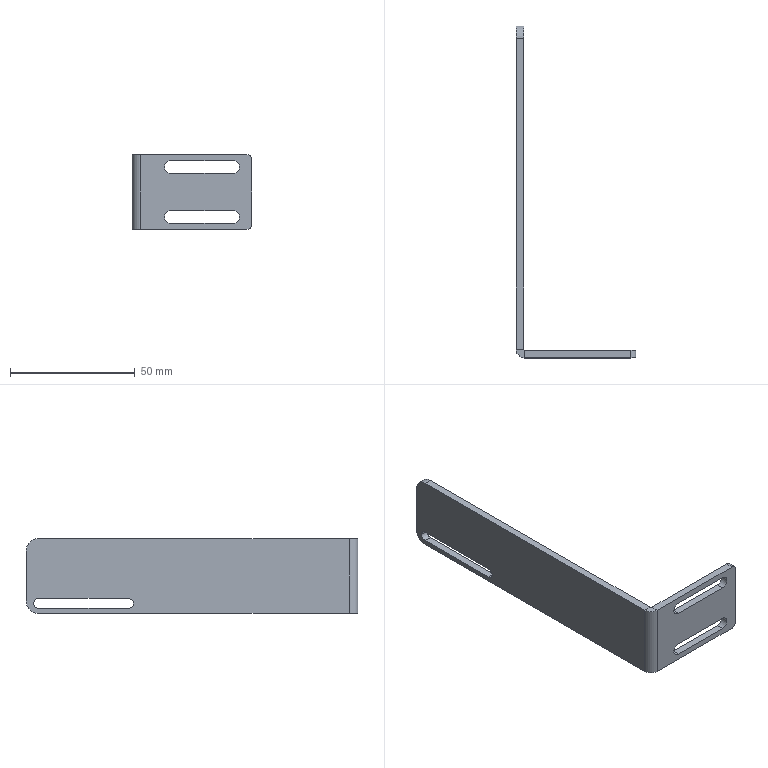Part | SolidWorks | features CornerTrim 2, ICE 2, FlatPattern 1, HoleWzd 1, SMBaseFlange 1, SheetMetal 1 | 1 solid | 31 faces | box 48 x 133 x 30 mm | volume 14568 mm3 | plane 18 | cylinder 13 | commonest cylinder face diameters 4 x5 5 x4 10 x2 1 x1 7 x1
STEP:
#1=CARTESIAN_POINT('',(-3.,127.,-11.));
#2=VERTEX_POINT('',#1);
#3=CARTESIAN_POINT('',(-3.,125.,-9.));
#4=VERTEX_POINT('',#3);
#5=CARTESIAN_POINT('',(-3.,125.,-11.));
#6=DIRECTION('',(1.,0.,0.));
#7=DIRECTION('',(0.,1.,0.));
#8=AXIS2_PLACEMENT_3D('',#5,#6,#7);
#9=CIRCLE('',#8,2.);
#10=EDGE_CURVE('',#2,#4,#9,.T.);
#11=ORIENTED_EDGE('',*,*,#10,.F.);
#12=CARTESIAN_POINT('',(0.,127.,-11.));
#13=VERTEX_POINT('',#12);
#14=CARTESIAN_POINT('',(-10.,127.,-11.));
#15=DIRECTION('',(1.,0.,0.));
#16=VECTOR('',#15,1000.);
#17=LINE('',#14,#16);
#18=EDGE_CURVE('',#2,#13,#17,.T.);
#19=ORIENTED_EDGE('',*,*,#18,.T.);
#20=CARTESIAN_POINT('',(0.,125.,-9.));
#21=VERTEX_POINT('',#20);
#22=CARTESIAN_POINT('',(0.,125.,-11.));
#23=DIRECTION('',(1.,0.,0.));
#24=DIRECTION('',(0.,1.,0.));
#25=AXIS2_PLACEMENT_3D('',#22,#23,#24);
#26=CIRCLE('',#25,2.);
#27=EDGE_CURVE('',#13,#21,#26,.T.);
#28=ORIENTED_EDGE('',*,*,#27,.T.);
#29=CARTESIAN_POINT('',(-10.,125.,-9.));
#30=DIRECTION('',(1.,0.,0.));
#31=VECTOR('',#30,1000.);
#32=LINE('',#29,#31);
#33=EDGE_CURVE('',#4,#21,#32,.T.);
#34=ORIENTED_EDGE('',*,*,#33,.F.);
#35=EDGE_LOOP('',(#11,#19,#28,#34));
#36=FACE_OUTER_BOUND('',#35,.T.);
#37=CARTESIAN_POINT('',(-10.,125.,-11.));
#38=DIRECTION('',(1.,0.,0.));
#39=DIRECTION('',(0.,1.,0.));
#40=AXIS2_PLACEMENT_3D('',#37,#38,#39);
#41=CYLINDRICAL_SURFACE('',#40,2.);
#42=ADVANCED_FACE('',(#36),#41,.F.);
#43=CARTESIAN_POINT('',(0.5,0.,15.));
#44=VERTEX_POINT('',#43);
#45=CARTESIAN_POINT('',(0.5,-3.,15.));
#46=VERTEX_POINT('',#45);
#47=CARTESIAN_POINT('',(0.5,0.,15.));
#48=DIRECTION('',(0.,-1.,0.));
#49=VECTOR('',#48,1000.);
#50=LINE('',#47,#49);
#51=EDGE_CURVE('',#44,#46,#50,.T.);
#52=ORIENTED_EDGE('',*,*,#51,.F.);
#53=CARTESIAN_POINT('',(0.,0.5,15.));
#54=VERTEX_POINT('',#53);
#55=CARTESIAN_POINT('',(0.5,0.5,15.));
#56=DIRECTION('',(0.,0.,1.));
#57=DIRECTION('',(-1.,0.,0.));
#58=AXIS2_PLACEMENT_3D('',#55,#56,#57);
#59=CIRCLE('',#58,0.5);
#60=EDGE_CURVE('',#54,#44,#59,.T.);
#61=ORIENTED_EDGE('',*,*,#60,.F.);
#62=CARTESIAN_POINT('',(-3.,0.5,15.));
#63=VERTEX_POINT('',#62);
#64=CARTESIAN_POINT('',(-3.,0.5,15.));
#65=DIRECTION('',(1.,0.,0.));
#66=VECTOR('',#65,1000.);
#67=LINE('',#64,#66);
#68=EDGE_CURVE('',#63,#54,#67,.T.);
#69=ORIENTED_EDGE('',*,*,#68,.F.);
#70=CARTESIAN_POINT('',(0.5,0.5,15.));
#71=DIRECTION('',(0.,0.,1.));
#72=DIRECTION('',(1.,0.,0.));
#73=AXIS2_PLACEMENT_3D('',#70,#71,#72);
#74=CIRCLE('',#73,3.5);
#75=EDGE_CURVE('',#63,#46,#74,.T.);
#76=ORIENTED_EDGE('',*,*,#75,.T.);
#77=EDGE_LOOP('',(#52,#61,#69,#76));
#78=FACE_OUTER_BOUND('',#77,.T.);
#79=CARTESIAN_POINT('',(0.5,0.,15.));
#80=DIRECTION('',(0.,0.,1.));
#81=DIRECTION('',(1.,0.,0.));
#82=AXIS2_PLACEMENT_3D('',#79,#80,#81);
#83=PLANE('',#82);
#84=ADVANCED_FACE('',(#78),#83,.T.);
#85=CARTESIAN_POINT('',(43.,-3.,15.));
#86=VERTEX_POINT('',#85);
#87=CARTESIAN_POINT('',(0.,-3.,15.));
#88=DIRECTION('',(1.,0.,0.));
#89=VECTOR('',#88,1000.);
#90=LINE('',#87,#89);
#91=EDGE_CURVE('',#46,#86,#90,.T.);
#92=ORIENTED_EDGE('',*,*,#91,.T.);
#93=CARTESIAN_POINT('',(43.,0.,15.));
#94=VERTEX_POINT('',#93);
#95=CARTESIAN_POINT('',(43.,0.5,15.));
#96=DIRECTION('',(0.,1.,0.));
#97=VECTOR('',#96,1000.);
#98=LINE('',#95,#97);
#99=EDGE_CURVE('',#86,#94,#98,.T.);
#100=ORIENTED_EDGE('',*,*,#99,.T.);
#101=CARTESIAN_POINT('',(0.,0.,15.));
#102=DIRECTION('',(1.,0.,0.));
#103=VECTOR('',#102,1000.);
#104=LINE('',#101,#103);
#105=EDGE_CURVE('',#44,#94,#104,.T.);
#106=ORIENTED_EDGE('',*,*,#105,.F.);
#107=ORIENTED_EDGE('',*,*,#51,.T.);
#108=EDGE_LOOP('',(#92,#100,#106,#107));
#109=FACE_OUTER_BOUND('',#108,.T.);
#110=CARTESIAN_POINT('',(-3.,0.5,15.));
#111=DIRECTION('',(0.,0.,1.));
#112=DIRECTION('',(1.,0.,0.));
#113=AXIS2_PLACEMENT_3D('',#110,#111,#112);
#114=PLANE('',#113);
#115=ADVANCED_FACE('',(#109),#114,.T.);
#116=CARTESIAN_POINT('',(0.,0.5,-15.));
#117=VERTEX_POINT('',#116);
#118=CARTESIAN_POINT('',(-3.,0.5,-15.));
#119=VERTEX_POINT('',#118);
#120=CARTESIAN_POINT('',(0.,0.5,-15.));
#121=DIRECTION('',(-1.,0.,0.));
#122=VECTOR('',#121,1000.);
#123=LINE('',#120,#122);
#124=EDGE_CURVE('',#117,#119,#123,.T.);
#125=ORIENTED_EDGE('',*,*,#124,.F.);
#126=CARTESIAN_POINT('',(0.5,0.,-15.));
#127=VERTEX_POINT('',#126);
#128=CARTESIAN_POINT('',(0.5,0.5,-15.));
#129=DIRECTION('',(0.,0.,1.));
#130=DIRECTION('',(-1.,0.,0.));
#131=AXIS2_PLACEMENT_3D('',#128,#129,#130);
#132=CIRCLE('',#131,0.5);
#133=EDGE_CURVE('',#117,#127,#132,.T.);
#134=ORIENTED_EDGE('',*,*,#133,.T.);
#135=CARTESIAN_POINT('',(0.5,-3.,-15.));
#136=VERTEX_POINT('',#135);
#137=CARTESIAN_POINT('',(0.5,-3.,-15.));
#138=DIRECTION('',(0.,1.,0.));
#139=VECTOR('',#138,1000.);
#140=LINE('',#137,#139);
#141=EDGE_CURVE('',#136,#127,#140,.T.);
#142=ORIENTED_EDGE('',*,*,#141,.F.);
#143=CARTESIAN_POINT('',(0.5,0.5,-15.));
#144=DIRECTION('',(0.,0.,1.));
#145=DIRECTION('',(1.,0.,0.));
#146=AXIS2_PLACEMENT_3D('',#143,#144,#145);
#147=CIRCLE('',#146,3.5);
#148=EDGE_CURVE('',#119,#136,#147,.T.);
#149=ORIENTED_EDGE('',*,*,#148,.F.);
#150=EDGE_LOOP('',(#125,#134,#142,#149));
#151=FACE_OUTER_BOUND('',#150,.T.);
#152=CARTESIAN_POINT('',(0.,0.5,-15.));
#153=DIRECTION('',(0.,0.,-1.));
#154=DIRECTION('',(-1.,0.,0.));
#155=AXIS2_PLACEMENT_3D('',#152,#153,#154);
#156=PLANE('',#155);
#157=ADVANCED_FACE('',(#151),#156,.T.);
#158=CARTESIAN_POINT('',(-3.,125.,-15.));
#159=VERTEX_POINT('',#158);
#160=CARTESIAN_POINT('',(-3.,130.,-15.));
#161=DIRECTION('',(0.,-1.,0.));
#162=VECTOR('',#161,1000.);
#163=LINE('',#160,#162);
#164=EDGE_CURVE('',#159,#119,#163,.T.);
#165=ORIENTED_EDGE('',*,*,#164,.F.);
#166=CARTESIAN_POINT('',(0.,125.,-15.));
#167=VERTEX_POINT('',#166);
#168=CARTESIAN_POINT('',(0.5,125.,-15.));
#169=DIRECTION('',(1.,0.,0.));
#170=VECTOR('',#169,1000.);
#171=LINE('',#168,#170);
#172=EDGE_CURVE('',#159,#167,#171,.T.);
#173=ORIENTED_EDGE('',*,*,#172,.T.);
#174=CARTESIAN_POINT('',(0.,130.,-15.));
#175=DIRECTION('',(0.,-1.,0.));
#176=VECTOR('',#175,1000.);
#177=LINE('',#174,#176);
#178=EDGE_CURVE('',#167,#117,#177,.T.);
#179=ORIENTED_EDGE('',*,*,#178,.T.);
#180=ORIENTED_EDGE('',*,*,#124,.T.);
#181=EDGE_LOOP('',(#165,#173,#179,#180));
#182=FACE_OUTER_BOUND('',#181,.T.);
#183=CARTESIAN_POINT('',(0.5,-3.,-15.));
#184=DIRECTION('',(0.,0.,-1.));
#185=DIRECTION('',(-1.,0.,0.));
#186=AXIS2_PLACEMENT_3D('',#183,#184,#185);
#187=PLANE('',#186);
#188=ADVANCED_FACE('',(#182),#187,.T.);
#189=CARTESIAN_POINT('',(37.5,-3.,7.5));
#190=VERTEX_POINT('',#189);
#191=CARTESIAN_POINT('',(12.5,-3.,7.5));
#192=VERTEX_POINT('',#191);
#193=CARTESIAN_POINT('',(0.,-3.,7.5));
#194=DIRECTION('',(-1.,0.,0.));
#195=VECTOR('',#194,1000.);
#196=LINE('',#193,#195);
#197=EDGE_CURVE('',#190,#192,#196,.T.);
#198=ORIENTED_EDGE('',*,*,#197,.T.);
#199=CARTESIAN_POINT('',(12.5,-3.,12.5));
#200=VERTEX_POINT('',#199);
#201=CARTESIAN_POINT('',(12.5,-3.,10.));
#202=DIRECTION('',(0.,1.,0.));
#203=DIRECTION('',(0.,0.,1.));
#204=AXIS2_PLACEMENT_3D('',#201,#202,#203);
#205=CIRCLE('',#204,2.5);
#206=EDGE_CURVE('',#192,#200,#205,.T.);
#207=ORIENTED_EDGE('',*,*,#206,.T.);
#208=CARTESIAN_POINT('',(37.5,-3.,12.5));
#209=VERTEX_POINT('',#208);
#210=CARTESIAN_POINT('',(0.,-3.,12.5));
#211=DIRECTION('',(1.,0.,0.));
#212=VECTOR('',#211,1000.);
#213=LINE('',#210,#212);
#214=EDGE_CURVE('',#200,#209,#213,.T.);
#215=ORIENTED_EDGE('',*,*,#214,.T.);
#216=CARTESIAN_POINT('',(37.5,-3.,10.));
#217=DIRECTION('',(0.,1.,0.));
#218=DIRECTION('',(0.,0.,1.));
#219=AXIS2_PLACEMENT_3D('',#216,#217,#218);
#220=CIRCLE('',#219,2.5);
#221=EDGE_CURVE('',#209,#190,#220,.T.);
#222=ORIENTED_EDGE('',*,*,#221,.T.);
#223=EDGE_LOOP('',(#198,#207,#215,#222));
#224=FACE_BOUND('',#223,.T.);
#225=CARTESIAN_POINT('',(37.5,-3.,-12.5));
#226=VERTEX_POINT('',#225);
#227=CARTESIAN_POINT('',(12.5,-3.,-12.5));
#228=VERTEX_POINT('',#227);
#229=CARTESIAN_POINT('',(0.,-3.,-12.5));
#230=DIRECTION('',(-1.,0.,0.));
#231=VECTOR('',#230,1000.);
#232=LINE('',#229,#231);
#233=EDGE_CURVE('',#226,#228,#232,.T.);
#234=ORIENTED_EDGE('',*,*,#233,.T.);
#235=CARTESIAN_POINT('',(12.5,-3.,-7.5));
#236=VERTEX_POINT('',#235);
#237=CARTESIAN_POINT('',(12.5,-3.,-10.));
#238=DIRECTION('',(0.,1.,0.));
#239=DIRECTION('',(0.,0.,1.));
#240=AXIS2_PLACEMENT_3D('',#237,#238,#239);
#241=CIRCLE('',#240,2.5);
#242=EDGE_CURVE('',#228,#236,#241,.T.);
#243=ORIENTED_EDGE('',*,*,#242,.T.);
#244=CARTESIAN_POINT('',(37.5,-3.,-7.5));
#245=VERTEX_POINT('',#244);
#246=CARTESIAN_POINT('',(0.,-3.,-7.5));
#247=DIRECTION('',(1.,0.,0.));
#248=VECTOR('',#247,1000.);
#249=LINE('',#246,#248);
#250=EDGE_CURVE('',#236,#245,#249,.T.);
#251=ORIENTED_EDGE('',*,*,#250,.T.);
#252=CARTESIAN_POINT('',(37.5,-3.,-10.));
#253=DIRECTION('',(0.,1.,0.));
#254=DIRECTION('',(0.,0.,1.));
#255=AXIS2_PLACEMENT_3D('',#252,#253,#254);
#256=CIRCLE('',#255,2.5);
#257=EDGE_CURVE('',#245,#226,#256,.T.);
#258=ORIENTED_EDGE('',*,*,#257,.T.);
#259=EDGE_LOOP('',(#234,#243,#251,#258));
#260=FACE_BOUND('',#259,.T.);
#261=CARTESIAN_POINT('',(43.,-3.,-15.));
#262=VERTEX_POINT('',#261);
#263=CARTESIAN_POINT('',(0.,-3.,-15.));
#264=DIRECTION('',(1.,0.,0.));
#265=VECTOR('',#264,1000.);
#266=LINE('',#263,#265);
#267=EDGE_CURVE('',#136,#262,#266,.T.);
#268=ORIENTED_EDGE('',*,*,#267,.T.);
#269=CARTESIAN_POINT('',(45.,-3.,-13.));
#270=VERTEX_POINT('',#269);
#271=CARTESIAN_POINT('',(43.,-3.,-13.));
#272=DIRECTION('',(0.,-1.,0.));
#273=DIRECTION('',(0.,0.,1.));
#274=AXIS2_PLACEMENT_3D('',#271,#272,#273);
#275=CIRCLE('',#274,2.);
#276=EDGE_CURVE('',#262,#270,#275,.T.);
#277=ORIENTED_EDGE('',*,*,#276,.T.);
#278=CARTESIAN_POINT('',(45.,-3.,13.));
#279=VERTEX_POINT('',#278);
#280=CARTESIAN_POINT('',(45.,-3.,15.));
#281=DIRECTION('',(0.,0.,-1.));
#282=VECTOR('',#281,1000.);
#283=LINE('',#280,#282);
#284=EDGE_CURVE('',#279,#270,#283,.T.);
#285=ORIENTED_EDGE('',*,*,#284,.F.);
#286=CARTESIAN_POINT('',(43.,-3.,13.));
#287=DIRECTION('',(0.,-1.,0.));
#288=DIRECTION('',(0.,0.,1.));
#289=AXIS2_PLACEMENT_3D('',#286,#287,#288);
#290=CIRCLE('',#289,2.);
#291=EDGE_CURVE('',#279,#86,#290,.T.);
#292=ORIENTED_EDGE('',*,*,#291,.T.);
#293=ORIENTED_EDGE('',*,*,#91,.F.);
#294=CARTESIAN_POINT('',(0.5,-3.,15.));
#295=DIRECTION('',(0.,0.,-1.));
#296=VECTOR('',#295,1000.);
#297=LINE('',#294,#296);
#298=EDGE_CURVE('',#46,#136,#297,.T.);
#299=ORIENTED_EDGE('',*,*,#298,.T.);
#300=EDGE_LOOP('',(#268,#277,#285,#292,#293,#299));
#301=FACE_OUTER_BOUND('',#300,.T.);
#302=CARTESIAN_POINT('',(0.,-3.,15.));
#303=DIRECTION('',(0.,1.,0.));
#304=DIRECTION('',(0.,0.,1.));
#305=AXIS2_PLACEMENT_3D('',#302,#303,#304);
#306=PLANE('',#305);
#307=ADVANCED_FACE('',(#224,#260,#301),#306,.F.);
#308=ORIENTED_EDGE('',*,*,#284,.T.);
#309=CARTESIAN_POINT('',(45.,0.,-13.));
#310=VERTEX_POINT('',#309);
#311=CARTESIAN_POINT('',(45.,0.,-13.));
#312=DIRECTION('',(0.,1.,0.));
#313=VECTOR('',#312,1000.);
#314=LINE('',#311,#313);
#315=EDGE_CURVE('',#270,#310,#314,.T.);
#316=ORIENTED_EDGE('',*,*,#315,.T.);
#317=CARTESIAN_POINT('',(45.,0.,13.));
#318=VERTEX_POINT('',#317);
#319=CARTESIAN_POINT('',(45.,0.,15.));
#320=DIRECTION('',(0.,0.,-1.));
#321=VECTOR('',#320,1000.);
#322=LINE('',#319,#321);
#323=EDGE_CURVE('',#318,#310,#322,.T.);
#324=ORIENTED_EDGE('',*,*,#323,.F.);
#325=CARTESIAN_POINT('',(45.,0.,13.));
#326=DIRECTION('',(0.,-1.,0.));
#327=VECTOR('',#326,1000.);
#328=LINE('',#325,#327);
#329=EDGE_CURVE('',#318,#279,#328,.T.);
#330=ORIENTED_EDGE('',*,*,#329,.T.);
#331=EDGE_LOOP('',(#308,#316,#324,#330));
#332=FACE_OUTER_BOUND('',#331,.T.);
#333=CARTESIAN_POINT('',(45.,0.,15.));
#334=DIRECTION('',(1.,0.,0.));
#335=DIRECTION('',(0.,0.,-1.));
#336=AXIS2_PLACEMENT_3D('',#333,#334,#335);
#337=PLANE('',#336);
#338=ADVANCED_FACE('',(#332),#337,.T.);
#339=CARTESIAN_POINT('',(12.5,0.,7.5));
#340=VERTEX_POINT('',#339);
#341=CARTESIAN_POINT('',(12.5,0.,12.5));
#342=VERTEX_POINT('',#341);
#343=CARTESIAN_POINT('',(12.5,0.,10.));
#344=DIRECTION('',(0.,1.,0.));
#345=DIRECTION('',(0.,0.,1.));
#346=AXIS2_PLACEMENT_3D('',#343,#344,#345);
#347=CIRCLE('',#346,2.5);
#348=EDGE_CURVE('',#340,#342,#347,.T.);
#349=ORIENTED_EDGE('',*,*,#348,.F.);
#350=CARTESIAN_POINT('',(37.5,0.,7.5));
#351=VERTEX_POINT('',#350);
#352=CARTESIAN_POINT('',(12.5,0.,7.5));
#353=DIRECTION('',(-1.,0.,0.));
#354=VECTOR('',#353,1000.);
#355=LINE('',#352,#354);
#356=EDGE_CURVE('',#351,#340,#355,.T.);
#357=ORIENTED_EDGE('',*,*,#356,.F.);
#358=CARTESIAN_POINT('',(37.5,0.,12.5));
#359=VERTEX_POINT('',#358);
#360=CARTESIAN_POINT('',(37.5,0.,10.));
#361=DIRECTION('',(0.,1.,0.));
#362=DIRECTION('',(0.,0.,1.));
#363=AXIS2_PLACEMENT_3D('',#360,#361,#362);
#364=CIRCLE('',#363,2.5);
#365=EDGE_CURVE('',#359,#351,#364,.T.);
#366=ORIENTED_EDGE('',*,*,#365,.F.);
#367=CARTESIAN_POINT('',(12.5,0.,12.5));
#368=DIRECTION('',(1.,0.,0.));
#369=VECTOR('',#368,1000.);
#370=LINE('',#367,#369);
#371=EDGE_CURVE('',#342,#359,#370,.T.);
#372=ORIENTED_EDGE('',*,*,#371,.F.);
#373=EDGE_LOOP('',(#349,#357,#366,#372));
#374=FACE_BOUND('',#373,.T.);
#375=CARTESIAN_POINT('',(12.5,0.,-12.5));
#376=VERTEX_POINT('',#375);
#377=CARTESIAN_POINT('',(12.5,0.,-7.5));
#378=VERTEX_POINT('',#377);
#379=CARTESIAN_POINT('',(12.5,0.,-10.));
#380=DIRECTION('',(0.,1.,0.));
#381=DIRECTION('',(0.,0.,1.));
#382=AXIS2_PLACEMENT_3D('',#379,#380,#381);
#383=CIRCLE('',#382,2.5);
#384=EDGE_CURVE('',#376,#378,#383,.T.);
#385=ORIENTED_EDGE('',*,*,#384,.F.);
#386=CARTESIAN_POINT('',(37.5,0.,-12.5));
#387=VERTEX_POINT('',#386);
#388=CARTESIAN_POINT('',(12.5,0.,-12.5));
#389=DIRECTION('',(-1.,0.,0.));
#390=VECTOR('',#389,1000.);
#391=LINE('',#388,#390);
#392=EDGE_CURVE('',#387,#376,#391,.T.);
#393=ORIENTED_EDGE('',*,*,#392,.F.);
#394=CARTESIAN_POINT('',(37.5,0.,-7.5));
#395=VERTEX_POINT('',#394);
#396=CARTESIAN_POINT('',(37.5,0.,-10.));
#397=DIRECTION('',(0.,1.,0.));
#398=DIRECTION('',(0.,0.,1.));
#399=AXIS2_PLACEMENT_3D('',#396,#397,#398);
#400=CIRCLE('',#399,2.5);
#401=EDGE_CURVE('',#395,#387,#400,.T.);
#402=ORIENTED_EDGE('',*,*,#401,.F.);
#403=CARTESIAN_POINT('',(12.5,0.,-7.5));
#404=DIRECTION('',(1.,0.,0.));
#405=VECTOR('',#404,1000.);
#406=LINE('',#403,#405);
#407=EDGE_CURVE('',#378,#395,#406,.T.);
#408=ORIENTED_EDGE('',*,*,#407,.F.);
#409=EDGE_LOOP('',(#385,#393,#402,#408));
#410=FACE_BOUND('',#409,.T.);
#411=ORIENTED_EDGE('',*,*,#323,.T.);
#412=CARTESIAN_POINT('',(43.,0.,-15.));
#413=VERTEX_POINT('',#412);
#414=CARTESIAN_POINT('',(43.,0.,-13.));
#415=DIRECTION('',(0.,1.,0.));
#416=DIRECTION('',(0.,0.,1.));
#417=AXIS2_PLACEMENT_3D('',#414,#415,#416);
#418=CIRCLE('',#417,2.);
#419=EDGE_CURVE('',#310,#413,#418,.T.);
#420=ORIENTED_EDGE('',*,*,#419,.T.);
#421=CARTESIAN_POINT('',(0.,0.,-15.));
#422=DIRECTION('',(1.,0.,0.));
#423=VECTOR('',#422,1000.);
#424=LINE('',#421,#423);
#425=EDGE_CURVE('',#127,#413,#424,.T.);
#426=ORIENTED_EDGE('',*,*,#425,.F.);
#427=CARTESIAN_POINT('',(0.5,0.,15.));
#428=DIRECTION('',(0.,0.,-1.));
#429=VECTOR('',#428,1000.);
#430=LINE('',#427,#429);
#431=EDGE_CURVE('',#44,#127,#430,.T.);
#432=ORIENTED_EDGE('',*,*,#431,.F.);
#433=ORIENTED_EDGE('',*,*,#105,.T.);
#434=CARTESIAN_POINT('',(43.,0.,13.));
#435=DIRECTION('',(0.,1.,0.));
#436=DIRECTION('',(0.,0.,1.));
#437=AXIS2_PLACEMENT_3D('',#434,#435,#436);
#438=CIRCLE('',#437,2.);
#439=EDGE_CURVE('',#94,#318,#438,.T.);
#440=ORIENTED_EDGE('',*,*,#439,.T.);
#441=EDGE_LOOP('',(#411,#420,#426,#432,#433,#440));
#442=FACE_OUTER_BOUND('',#441,.T.);
#443=CARTESIAN_POINT('',(0.,0.,15.));
#444=DIRECTION('',(0.,1.,0.));
#445=DIRECTION('',(0.,0.,1.));
#446=AXIS2_PLACEMENT_3D('',#443,#444,#445);
#447=PLANE('',#446);
#448=ADVANCED_FACE('',(#374,#410,#442),#447,.T.);
#449=ORIENTED_EDGE('',*,*,#133,.F.);
#450=CARTESIAN_POINT('',(0.,0.5,15.));
#451=DIRECTION('',(0.,0.,-1.));
#452=VECTOR('',#451,1000.);
#453=LINE('',#450,#452);
#454=EDGE_CURVE('',#54,#117,#453,.T.);
#455=ORIENTED_EDGE('',*,*,#454,.F.);
#456=ORIENTED_EDGE('',*,*,#60,.T.);
#457=ORIENTED_EDGE('',*,*,#431,.T.);
#458=EDGE_LOOP('',(#449,#455,#456,#457));
#459=FACE_OUTER_BOUND('',#458,.T.);
#460=CARTESIAN_POINT('',(0.5,0.5,15.));
#461=DIRECTION('',(0.,0.,-1.));
#462=DIRECTION('',(-1.,0.,0.));
#463=AXIS2_PLACEMENT_3D('',#460,#461,#462);
#464=CYLINDRICAL_SURFACE('',#463,0.5);
#465=ADVANCED_FACE('',(#459),#464,.F.);
#466=CARTESIAN_POINT('',(0.,89.,-9.));
#467=VERTEX_POINT('',#466);
#468=CARTESIAN_POINT('',(0.,89.,-13.));
#469=VERTEX_POINT('',#468);
#470=CARTESIAN_POINT('',(0.,89.,-11.));
#471=DIRECTION('',(1.,0.,0.));
#472=DIRECTION('',(0.,1.,0.));
#473=AXIS2_PLACEMENT_3D('',#470,#471,#472);
#474=CIRCLE('',#473,2.);
#475=EDGE_CURVE('',#467,#469,#474,.T.);
#476=ORIENTED_EDGE('',*,*,#475,.F.);
#477=CARTESIAN_POINT('',(0.,89.,-9.));
#478=DIRECTION('',(0.,-1.,0.));
#479=VECTOR('',#478,1000.);
#480=LINE('',#477,#479);
#481=EDGE_CURVE('',#21,#467,#480,.T.);
#482=ORIENTED_EDGE('',*,*,#481,.F.);
#483=ORIENTED_EDGE('',*,*,#27,.F.);
#484=CARTESIAN_POINT('',(0.,125.,-13.));
#485=VERTEX_POINT('',#484);
#486=CARTESIAN_POINT('',(0.,125.,-11.));
#487=DIRECTION('',(1.,0.,0.));
#488=DIRECTION('',(0.,1.,0.));
#489=AXIS2_PLACEMENT_3D('',#486,#487,#488);
#490=CIRCLE('',#489,2.);
#491=EDGE_CURVE('',#485,#13,#490,.T.);
#492=ORIENTED_EDGE('',*,*,#491,.F.);
#493=CARTESIAN_POINT('',(0.,89.,-13.));
#494=DIRECTION('',(0.,1.,0.));
#495=VECTOR('',#494,1000.);
#496=LINE('',#493,#495);
#497=EDGE_CURVE('',#469,#485,#496,.T.);
#498=ORIENTED_EDGE('',*,*,#497,.F.);
#499=EDGE_LOOP('',(#476,#482,#483,#492,#498));
#500=FACE_BOUND('',#499,.T.);
#501=ORIENTED_EDGE('',*,*,#178,.F.);
#502=CARTESIAN_POINT('',(0.,130.,-10.));
#503=VERTEX_POINT('',#502);
#504=CARTESIAN_POINT('',(0.,125.,-10.));
#505=DIRECTION('',(1.,0.,0.));
#506=DIRECTION('',(0.,1.,0.));
#507=AXIS2_PLACEMENT_3D('',#504,#505,#506);
#508=CIRCLE('',#507,5.);
#509=EDGE_CURVE('',#167,#503,#508,.T.);
#510=ORIENTED_EDGE('',*,*,#509,.T.);
#511=CARTESIAN_POINT('',(0.,130.,10.));
#512=VERTEX_POINT('',#511);
#513=CARTESIAN_POINT('',(0.,130.,15.));
#514=DIRECTION('',(0.,0.,-1.));
#515=VECTOR('',#514,1000.);
#516=LINE('',#513,#515);
#517=EDGE_CURVE('',#512,#503,#516,.T.);
#518=ORIENTED_EDGE('',*,*,#517,.F.);
#519=CARTESIAN_POINT('',(0.,125.,15.));
#520=VERTEX_POINT('',#519);
#521=CARTESIAN_POINT('',(0.,125.,10.));
#522=DIRECTION('',(1.,0.,0.));
#523=DIRECTION('',(0.,1.,0.));
#524=AXIS2_PLACEMENT_3D('',#521,#522,#523);
#525=CIRCLE('',#524,5.);
#526=EDGE_CURVE('',#512,#520,#525,.T.);
#527=ORIENTED_EDGE('',*,*,#526,.T.);
#528=CARTESIAN_POINT('',(0.,130.,15.));
#529=DIRECTION('',(0.,-1.,0.));
#530=VECTOR('',#529,1000.);
#531=LINE('',#528,#530);
#532=EDGE_CURVE('',#520,#54,#531,.T.);
#533=ORIENTED_EDGE('',*,*,#532,.T.);
#534=ORIENTED_EDGE('',*,*,#454,.T.);
#535=EDGE_LOOP('',(#501,#510,#518,#527,#533,#534));
#536=FACE_OUTER_BOUND('',#535,.T.);
#537=CARTESIAN_POINT('',(0.,130.,15.));
#538=DIRECTION('',(1.,0.,0.));
#539=DIRECTION('',(0.,1.,0.));
#540=AXIS2_PLACEMENT_3D('',#537,#538,#539);
#541=PLANE('',#540);
#542=ADVANCED_FACE('',(#500,#536),#541,.T.);
#543=ORIENTED_EDGE('',*,*,#517,.T.);
#544=CARTESIAN_POINT('',(-3.,130.,-10.));
#545=VERTEX_POINT('',#544);
#546=CARTESIAN_POINT('',(-3.,130.,-10.));
#547=DIRECTION('',(-1.,0.,0.));
#548=VECTOR('',#547,1000.);
#549=LINE('',#546,#548);
#550=EDGE_CURVE('',#503,#545,#549,.T.);
#551=ORIENTED_EDGE('',*,*,#550,.T.);
#552=CARTESIAN_POINT('',(-3.,130.,10.));
#553=VERTEX_POINT('',#552);
#554=CARTESIAN_POINT('',(-3.,130.,15.));
#555=DIRECTION('',(0.,0.,-1.));
#556=VECTOR('',#555,1000.);
#557=LINE('',#554,#556);
#558=EDGE_CURVE('',#553,#545,#557,.T.);
#559=ORIENTED_EDGE('',*,*,#558,.F.);
#560=CARTESIAN_POINT('',(0.,130.,10.));
#561=DIRECTION('',(1.,0.,0.));
#562=VECTOR('',#561,1000.);
#563=LINE('',#560,#562);
#564=EDGE_CURVE('',#553,#512,#563,.T.);
#565=ORIENTED_EDGE('',*,*,#564,.T.);
#566=EDGE_LOOP('',(#543,#551,#559,#565));
#567=FACE_OUTER_BOUND('',#566,.T.);
#568=CARTESIAN_POINT('',(-3.,130.,15.));
#569=DIRECTION('',(0.,1.,0.));
#570=DIRECTION('',(0.,0.,1.));
#571=AXIS2_PLACEMENT_3D('',#568,#569,#570);
#572=PLANE('',#571);
#573=ADVANCED_FACE('',(#567),#572,.T.);
#574=CARTESIAN_POINT('',(-3.,89.,-9.));
#575=VERTEX_POINT('',#574);
#576=CARTESIAN_POINT('',(-3.,130.,-9.));
#577=DIRECTION('',(0.,-1.,0.));
#578=VECTOR('',#577,1000.);
#579=LINE('',#576,#578);
#580=EDGE_CURVE('',#4,#575,#579,.T.);
#581=ORIENTED_EDGE('',*,*,#580,.T.);
#582=CARTESIAN_POINT('',(-3.,89.,-13.));
#583=VERTEX_POINT('',#582);
#584=CARTESIAN_POINT('',(-3.,89.,-11.));
#585=DIRECTION('',(1.,0.,0.));
#586=DIRECTION('',(0.,1.,0.));
#587=AXIS2_PLACEMENT_3D('',#584,#585,#586);
#588=CIRCLE('',#587,2.);
#589=EDGE_CURVE('',#575,#583,#588,.T.);
#590=ORIENTED_EDGE('',*,*,#589,.T.);
#591=CARTESIAN_POINT('',(-3.,125.,-13.));
#592=VERTEX_POINT('',#591);
#593=CARTESIAN_POINT('',(-3.,130.,-13.));
#594=DIRECTION('',(0.,1.,0.));
#595=VECTOR('',#594,1000.);
#596=LINE('',#593,#595);
#597=EDGE_CURVE('',#583,#592,#596,.T.);
#598=ORIENTED_EDGE('',*,*,#597,.T.);
#599=CARTESIAN_POINT('',(-3.,125.,-11.));
#600=DIRECTION('',(1.,0.,0.));
#601=DIRECTION('',(0.,1.,0.));
#602=AXIS2_PLACEMENT_3D('',#599,#600,#601);
#603=CIRCLE('',#602,2.);
#604=EDGE_CURVE('',#592,#2,#603,.T.);
#605=ORIENTED_EDGE('',*,*,#604,.T.);
#606=ORIENTED_EDGE('',*,*,#10,.T.);
#607=EDGE_LOOP('',(#581,#590,#598,#605,#606));
#608=FACE_BOUND('',#607,.T.);
#609=ORIENTED_EDGE('',*,*,#558,.T.);
#610=CARTESIAN_POINT('',(-3.,125.,-10.));
#611=DIRECTION('',(-1.,0.,0.));
#612=DIRECTION('',(0.,1.,0.));
#613=AXIS2_PLACEMENT_3D('',#610,#611,#612);
#614=CIRCLE('',#613,5.);
#615=EDGE_CURVE('',#545,#159,#614,.T.);
#616=ORIENTED_EDGE('',*,*,#615,.T.);
#617=ORIENTED_EDGE('',*,*,#164,.T.);
#618=CARTESIAN_POINT('',(-3.,0.5,15.));
#619=DIRECTION('',(0.,0.,-1.));
#620=VECTOR('',#619,1000.);
#621=LINE('',#618,#620);
#622=EDGE_CURVE('',#63,#119,#621,.T.);
#623=ORIENTED_EDGE('',*,*,#622,.F.);
#624=CARTESIAN_POINT('',(-3.,125.,15.));
#625=VERTEX_POINT('',#624);
#626=CARTESIAN_POINT('',(-3.,130.,15.));
#627=DIRECTION('',(0.,-1.,0.));
#628=VECTOR('',#627,1000.);
#629=LINE('',#626,#628);
#630=EDGE_CURVE('',#625,#63,#629,.T.);
#631=ORIENTED_EDGE('',*,*,#630,.F.);
#632=CARTESIAN_POINT('',(-3.,125.,10.));
#633=DIRECTION('',(-1.,0.,0.));
#634=DIRECTION('',(0.,1.,0.));
#635=AXIS2_PLACEMENT_3D('',#632,#633,#634);
#636=CIRCLE('',#635,5.);
#637=EDGE_CURVE('',#625,#553,#636,.T.);
#638=ORIENTED_EDGE('',*,*,#637,.T.);
#639=EDGE_LOOP('',(#609,#616,#617,#623,#631,#638));
#640=FACE_OUTER_BOUND('',#639,.T.);
#641=CARTESIAN_POINT('',(-3.,130.,15.));
#642=DIRECTION('',(1.,0.,0.));
#643=DIRECTION('',(0.,1.,0.));
#644=AXIS2_PLACEMENT_3D('',#641,#642,#643);
#645=PLANE('',#644);
#646=ADVANCED_FACE('',(#608,#640),#645,.F.);
#647=ORIENTED_EDGE('',*,*,#148,.T.);
#648=ORIENTED_EDGE('',*,*,#298,.F.);
#649=ORIENTED_EDGE('',*,*,#75,.F.);
#650=ORIENTED_EDGE('',*,*,#622,.T.);
#651=EDGE_LOOP('',(#647,#648,#649,#650));
#652=FACE_OUTER_BOUND('',#651,.T.);
#653=CARTESIAN_POINT('',(0.5,0.5,15.));
#654=DIRECTION('',(0.,0.,-1.));
#655=DIRECTION('',(-1.,0.,0.));
#656=AXIS2_PLACEMENT_3D('',#653,#654,#655);
#657=CYLINDRICAL_SURFACE('',#656,3.5);
#658=ADVANCED_FACE('',(#652),#657,.T.);
#659=ORIENTED_EDGE('',*,*,#532,.F.);
#660=CARTESIAN_POINT('',(-3.,125.,15.));
#661=DIRECTION('',(-1.,0.,0.));
#662=VECTOR('',#661,1000.);
#663=LINE('',#660,#662);
#664=EDGE_CURVE('',#520,#625,#663,.T.);
#665=ORIENTED_EDGE('',*,*,#664,.T.);
#666=ORIENTED_EDGE('',*,*,#630,.T.);
#667=ORIENTED_EDGE('',*,*,#68,.T.);
#668=EDGE_LOOP('',(#659,#665,#666,#667));
#669=FACE_OUTER_BOUND('',#668,.T.);
#670=CARTESIAN_POINT('',(0.5,0.5,15.));
#671=DIRECTION('',(0.,0.,-1.));
#672=DIRECTION('',(-1.,0.,0.));
#673=AXIS2_PLACEMENT_3D('',#670,#671,#672);
#674=PLANE('',#673);
#675=ADVANCED_FACE('',(#669),#674,.F.);
#676=ORIENTED_EDGE('',*,*,#425,.T.);
#677=CARTESIAN_POINT('',(43.,0.5,-15.));
#678=DIRECTION('',(0.,-1.,0.));
#679=VECTOR('',#678,1000.);
#680=LINE('',#677,#679);
#681=EDGE_CURVE('',#413,#262,#680,.T.);
#682=ORIENTED_EDGE('',*,*,#681,.T.);
#683=ORIENTED_EDGE('',*,*,#267,.F.);
#684=ORIENTED_EDGE('',*,*,#141,.T.);
#685=EDGE_LOOP('',(#676,#682,#683,#684));
#686=FACE_OUTER_BOUND('',#685,.T.);
#687=CARTESIAN_POINT('',(0.5,0.5,-15.));
#688=DIRECTION('',(0.,0.,-1.));
#689=DIRECTION('',(-1.,0.,0.));
#690=AXIS2_PLACEMENT_3D('',#687,#688,#689);
#691=PLANE('',#690);
#692=ADVANCED_FACE('',(#686),#691,.T.);
#693=ORIENTED_EDGE('',*,*,#615,.F.);
#694=ORIENTED_EDGE('',*,*,#550,.F.);
#695=ORIENTED_EDGE('',*,*,#509,.F.);
#696=ORIENTED_EDGE('',*,*,#172,.F.);
#697=EDGE_LOOP('',(#693,#694,#695,#696));
#698=FACE_OUTER_BOUND('',#697,.T.);
#699=CARTESIAN_POINT('',(0.5,125.,-10.));
#700=DIRECTION('',(1.,0.,0.));
#701=DIRECTION('',(0.,0.,-1.));
#702=AXIS2_PLACEMENT_3D('',#699,#700,#701);
#703=CYLINDRICAL_SURFACE('',#702,5.);
#704=ADVANCED_FACE('',(#698),#703,.T.);
#705=ORIENTED_EDGE('',*,*,#637,.F.);
#706=ORIENTED_EDGE('',*,*,#664,.F.);
#707=ORIENTED_EDGE('',*,*,#526,.F.);
#708=ORIENTED_EDGE('',*,*,#564,.F.);
#709=EDGE_LOOP('',(#705,#706,#707,#708));
#710=FACE_OUTER_BOUND('',#709,.T.);
#711=CARTESIAN_POINT('',(-3.,125.,10.));
#712=DIRECTION('',(-1.,0.,0.));
#713=DIRECTION('',(0.,0.,1.));
#714=AXIS2_PLACEMENT_3D('',#711,#712,#713);
#715=CYLINDRICAL_SURFACE('',#714,5.);
#716=ADVANCED_FACE('',(#710),#715,.T.);
#717=ORIENTED_EDGE('',*,*,#419,.F.);
#718=ORIENTED_EDGE('',*,*,#315,.F.);
#719=ORIENTED_EDGE('',*,*,#276,.F.);
#720=ORIENTED_EDGE('',*,*,#681,.F.);
#721=EDGE_LOOP('',(#717,#718,#719,#720));
#722=FACE_OUTER_BOUND('',#721,.T.);
#723=CARTESIAN_POINT('',(43.,0.5,-13.));
#724=DIRECTION('',(0.,-1.,0.));
#725=DIRECTION('',(0.,0.,-1.));
#726=AXIS2_PLACEMENT_3D('',#723,#724,#725);
#727=CYLINDRICAL_SURFACE('',#726,2.);
#728=ADVANCED_FACE('',(#722),#727,.T.);
#729=ORIENTED_EDGE('',*,*,#439,.F.);
#730=ORIENTED_EDGE('',*,*,#99,.F.);
#731=ORIENTED_EDGE('',*,*,#291,.F.);
#732=ORIENTED_EDGE('',*,*,#329,.F.);
#733=EDGE_LOOP('',(#729,#730,#731,#732));
#734=FACE_OUTER_BOUND('',#733,.T.);
#735=CARTESIAN_POINT('',(43.,0.,13.));
#736=DIRECTION('',(0.,-1.,0.));
#737=DIRECTION('',(0.,0.,-1.));
#738=AXIS2_PLACEMENT_3D('',#735,#736,#737);
#739=CYLINDRICAL_SURFACE('',#738,2.);
#740=ADVANCED_FACE('',(#734),#739,.T.);
#741=CARTESIAN_POINT('',(-10.,89.,-9.));
#742=DIRECTION('',(1.,0.,0.));
#743=VECTOR('',#742,1000.);
#744=LINE('',#741,#743);
#745=EDGE_CURVE('',#575,#467,#744,.T.);
#746=ORIENTED_EDGE('',*,*,#745,.T.);
#747=ORIENTED_EDGE('',*,*,#475,.T.);
#748=CARTESIAN_POINT('',(-10.,89.,-13.));
#749=DIRECTION('',(1.,0.,0.));
#750=VECTOR('',#749,1000.);
#751=LINE('',#748,#750);
#752=EDGE_CURVE('',#583,#469,#751,.T.);
#753=ORIENTED_EDGE('',*,*,#752,.F.);
#754=ORIENTED_EDGE('',*,*,#589,.F.);
#755=EDGE_LOOP('',(#746,#747,#753,#754));
#756=FACE_OUTER_BOUND('',#755,.T.);
#757=CARTESIAN_POINT('',(-10.,89.,-11.));
#758=DIRECTION('',(1.,0.,0.));
#759=DIRECTION('',(0.,1.,0.));
#760=AXIS2_PLACEMENT_3D('',#757,#758,#759);
#761=CYLINDRICAL_SURFACE('',#760,2.);
#762=ADVANCED_FACE('',(#756),#761,.F.);
#763=ORIENTED_EDGE('',*,*,#33,.T.);
#764=ORIENTED_EDGE('',*,*,#481,.T.);
#765=ORIENTED_EDGE('',*,*,#745,.F.);
#766=ORIENTED_EDGE('',*,*,#580,.F.);
#767=EDGE_LOOP('',(#763,#764,#765,#766));
#768=FACE_OUTER_BOUND('',#767,.T.);
#769=CARTESIAN_POINT('',(-10.,89.,-9.));
#770=DIRECTION('',(0.,0.,1.));
#771=DIRECTION('',(1.,0.,0.));
#772=AXIS2_PLACEMENT_3D('',#769,#770,#771);
#773=PLANE('',#772);
#774=ADVANCED_FACE('',(#768),#773,.F.);
#775=ORIENTED_EDGE('',*,*,#18,.F.);
#776=ORIENTED_EDGE('',*,*,#604,.F.);
#777=CARTESIAN_POINT('',(-10.,125.,-13.));
#778=DIRECTION('',(1.,0.,0.));
#779=VECTOR('',#778,1000.);
#780=LINE('',#777,#779);
#781=EDGE_CURVE('',#592,#485,#780,.T.);
#782=ORIENTED_EDGE('',*,*,#781,.T.);
#783=ORIENTED_EDGE('',*,*,#491,.T.);
#784=EDGE_LOOP('',(#775,#776,#782,#783));
#785=FACE_OUTER_BOUND('',#784,.T.);
#786=CARTESIAN_POINT('',(-10.,125.,-11.));
#787=DIRECTION('',(1.,0.,0.));
#788=DIRECTION('',(0.,1.,0.));
#789=AXIS2_PLACEMENT_3D('',#786,#787,#788);
#790=CYLINDRICAL_SURFACE('',#789,2.);
#791=ADVANCED_FACE('',(#785),#790,.F.);
#792=ORIENTED_EDGE('',*,*,#752,.T.);
#793=ORIENTED_EDGE('',*,*,#497,.T.);
#794=ORIENTED_EDGE('',*,*,#781,.F.);
#795=ORIENTED_EDGE('',*,*,#597,.F.);
#796=EDGE_LOOP('',(#792,#793,#794,#795));
#797=FACE_OUTER_BOUND('',#796,.T.);
#798=CARTESIAN_POINT('',(-10.,89.,-13.));
#799=DIRECTION('',(0.,0.,-1.));
#800=DIRECTION('',(-1.,0.,0.));
#801=AXIS2_PLACEMENT_3D('',#798,#799,#800);
#802=PLANE('',#801);
#803=ADVANCED_FACE('',(#797),#802,.F.);
#804=CARTESIAN_POINT('',(12.5,-10.,-12.5));
#805=DIRECTION('',(0.,1.,0.));
#806=VECTOR('',#805,1000.);
#807=LINE('',#804,#806);
#808=EDGE_CURVE('',#228,#376,#807,.T.);
#809=ORIENTED_EDGE('',*,*,#808,.T.);
#810=ORIENTED_EDGE('',*,*,#384,.T.);
#811=CARTESIAN_POINT('',(12.5,-10.,-7.5));
#812=DIRECTION('',(0.,1.,0.));
#813=VECTOR('',#812,1000.);
#814=LINE('',#811,#813);
#815=EDGE_CURVE('',#236,#378,#814,.T.);
#816=ORIENTED_EDGE('',*,*,#815,.F.);
#817=ORIENTED_EDGE('',*,*,#242,.F.);
#818=EDGE_LOOP('',(#809,#810,#816,#817));
#819=FACE_OUTER_BOUND('',#818,.T.);
#820=CARTESIAN_POINT('',(12.5,-10.,-10.));
#821=DIRECTION('',(0.,1.,0.));
#822=DIRECTION('',(0.,0.,1.));
#823=AXIS2_PLACEMENT_3D('',#820,#821,#822);
#824=CYLINDRICAL_SURFACE('',#823,2.5);
#825=ADVANCED_FACE('',(#819),#824,.F.);
#826=CARTESIAN_POINT('',(37.5,-10.,-12.5));
#827=DIRECTION('',(0.,1.,0.));
#828=VECTOR('',#827,1000.);
#829=LINE('',#826,#828);
#830=EDGE_CURVE('',#226,#387,#829,.T.);
#831=ORIENTED_EDGE('',*,*,#830,.T.);
#832=ORIENTED_EDGE('',*,*,#392,.T.);
#833=ORIENTED_EDGE('',*,*,#808,.F.);
#834=ORIENTED_EDGE('',*,*,#233,.F.);
#835=EDGE_LOOP('',(#831,#832,#833,#834));
#836=FACE_OUTER_BOUND('',#835,.T.);
#837=CARTESIAN_POINT('',(12.5,-10.,-12.5));
#838=DIRECTION('',(0.,0.,-1.));
#839=DIRECTION('',(-1.,0.,0.));
#840=AXIS2_PLACEMENT_3D('',#837,#838,#839);
#841=PLANE('',#840);
#842=ADVANCED_FACE('',(#836),#841,.F.);
#843=CARTESIAN_POINT('',(37.5,-10.,-7.5));
#844=DIRECTION('',(0.,1.,0.));
#845=VECTOR('',#844,1000.);
#846=LINE('',#843,#845);
#847=EDGE_CURVE('',#245,#395,#846,.T.);
#848=ORIENTED_EDGE('',*,*,#847,.T.);
#849=ORIENTED_EDGE('',*,*,#401,.T.);
#850=ORIENTED_EDGE('',*,*,#830,.F.);
#851=ORIENTED_EDGE('',*,*,#257,.F.);
#852=EDGE_LOOP('',(#848,#849,#850,#851));
#853=FACE_OUTER_BOUND('',#852,.T.);
#854=CARTESIAN_POINT('',(37.5,-10.,-10.));
#855=DIRECTION('',(0.,1.,0.));
#856=DIRECTION('',(0.,0.,1.));
#857=AXIS2_PLACEMENT_3D('',#854,#855,#856);
#858=CYLINDRICAL_SURFACE('',#857,2.5);
#859=ADVANCED_FACE('',(#853),#858,.F.);
#860=ORIENTED_EDGE('',*,*,#815,.T.);
#861=ORIENTED_EDGE('',*,*,#407,.T.);
#862=ORIENTED_EDGE('',*,*,#847,.F.);
#863=ORIENTED_EDGE('',*,*,#250,.F.);
#864=EDGE_LOOP('',(#860,#861,#862,#863));
#865=FACE_OUTER_BOUND('',#864,.T.);
#866=CARTESIAN_POINT('',(12.5,-10.,-7.5));
#867=DIRECTION('',(0.,0.,1.));
#868=DIRECTION('',(1.,0.,0.));
#869=AXIS2_PLACEMENT_3D('',#866,#867,#868);
#870=PLANE('',#869);
#871=ADVANCED_FACE('',(#865),#870,.F.);
#872=CARTESIAN_POINT('',(12.5,-10.,7.5));
#873=DIRECTION('',(0.,1.,0.));
#874=VECTOR('',#873,1000.);
#875=LINE('',#872,#874);
#876=EDGE_CURVE('',#192,#340,#875,.T.);
#877=ORIENTED_EDGE('',*,*,#876,.T.);
#878=ORIENTED_EDGE('',*,*,#348,.T.);
#879=CARTESIAN_POINT('',(12.5,-10.,12.5));
#880=DIRECTION('',(0.,1.,0.));
#881=VECTOR('',#880,1000.);
#882=LINE('',#879,#881);
#883=EDGE_CURVE('',#200,#342,#882,.T.);
#884=ORIENTED_EDGE('',*,*,#883,.F.);
#885=ORIENTED_EDGE('',*,*,#206,.F.);
#886=EDGE_LOOP('',(#877,#878,#884,#885));
#887=FACE_OUTER_BOUND('',#886,.T.);
#888=CARTESIAN_POINT('',(12.5,-10.,10.));
#889=DIRECTION('',(0.,1.,0.));
#890=DIRECTION('',(0.,0.,1.));
#891=AXIS2_PLACEMENT_3D('',#888,#889,#890);
#892=CYLINDRICAL_SURFACE('',#891,2.5);
#893=ADVANCED_FACE('',(#887),#892,.F.);
#894=CARTESIAN_POINT('',(37.5,-10.,7.5));
#895=DIRECTION('',(0.,1.,0.));
#896=VECTOR('',#895,1000.);
#897=LINE('',#894,#896);
#898=EDGE_CURVE('',#190,#351,#897,.T.);
#899=ORIENTED_EDGE('',*,*,#898,.T.);
#900=ORIENTED_EDGE('',*,*,#356,.T.);
#901=ORIENTED_EDGE('',*,*,#876,.F.);
#902=ORIENTED_EDGE('',*,*,#197,.F.);
#903=EDGE_LOOP('',(#899,#900,#901,#902));
#904=FACE_OUTER_BOUND('',#903,.T.);
#905=CARTESIAN_POINT('',(12.5,-10.,7.5));
#906=DIRECTION('',(0.,0.,-1.));
#907=DIRECTION('',(-1.,0.,0.));
#908=AXIS2_PLACEMENT_3D('',#905,#906,#907);
#909=PLANE('',#908);
#910=ADVANCED_FACE('',(#904),#909,.F.);
#911=CARTESIAN_POINT('',(37.5,-10.,12.5));
#912=DIRECTION('',(0.,1.,0.));
#913=VECTOR('',#912,1000.);
#914=LINE('',#911,#913);
#915=EDGE_CURVE('',#209,#359,#914,.T.);
#916=ORIENTED_EDGE('',*,*,#915,.T.);
#917=ORIENTED_EDGE('',*,*,#365,.T.);
#918=ORIENTED_EDGE('',*,*,#898,.F.);
#919=ORIENTED_EDGE('',*,*,#221,.F.);
#920=EDGE_LOOP('',(#916,#917,#918,#919));
#921=FACE_OUTER_BOUND('',#920,.T.);
#922=CARTESIAN_POINT('',(37.5,-10.,10.));
#923=DIRECTION('',(0.,1.,0.));
#924=DIRECTION('',(0.,0.,1.));
#925=AXIS2_PLACEMENT_3D('',#922,#923,#924);
#926=CYLINDRICAL_SURFACE('',#925,2.5);
#927=ADVANCED_FACE('',(#921),#926,.F.);
#928=ORIENTED_EDGE('',*,*,#883,.T.);
#929=ORIENTED_EDGE('',*,*,#371,.T.);
#930=ORIENTED_EDGE('',*,*,#915,.F.);
#931=ORIENTED_EDGE('',*,*,#214,.F.);
#932=EDGE_LOOP('',(#928,#929,#930,#931));
#933=FACE_OUTER_BOUND('',#932,.T.);
#934=CARTESIAN_POINT('',(12.5,-10.,12.5));
#935=DIRECTION('',(0.,0.,1.));
#936=DIRECTION('',(1.,0.,0.));
#937=AXIS2_PLACEMENT_3D('',#934,#935,#936);
#938=PLANE('',#937);
#939=ADVANCED_FACE('',(#933),#938,.F.);
#940=CLOSED_SHELL('',(#42,#84,#115,#157,#188,#307,#338,#448,#465,#542,#573,#646,#658,#675,#692,#704,#716,#728,#740,#762,#774,#791,#803,#825,#842,#859,#871,#893,#910,#927,#939));
#941=MANIFOLD_SOLID_BREP('',#940);
#942=CARTESIAN_POINT('',(0.,0.,0.));
#943=DIRECTION('',(0.,0.,1.));
#944=DIRECTION('',(1.,0.,0.));
#945=AXIS2_PLACEMENT_3D('',#942,#943,#944);
#946=(LENGTH_UNIT()NAMED_UNIT(*)SI_UNIT(.MILLI.,.METRE.));
#947=UNCERTAINTY_MEASURE_WITH_UNIT(LENGTH_MEASURE(0.00001),#946,'','');
#948=(NAMED_UNIT(*)PLANE_ANGLE_UNIT()SI_UNIT($,.RADIAN.));
#949=(NAMED_UNIT(*)SI_UNIT($,.STERADIAN.)SOLID_ANGLE_UNIT());
#950=(GEOMETRIC_REPRESENTATION_CONTEXT(3)GLOBAL_UNCERTAINTY_ASSIGNED_CONTEXT((#947))GLOBAL_UNIT_ASSIGNED_CONTEXT((#946,#948,#949))REPRESENTATION_CONTEXT('',''));
#951=ADVANCED_BREP_SHAPE_REPRESENTATION('',(#941,#945),#950);